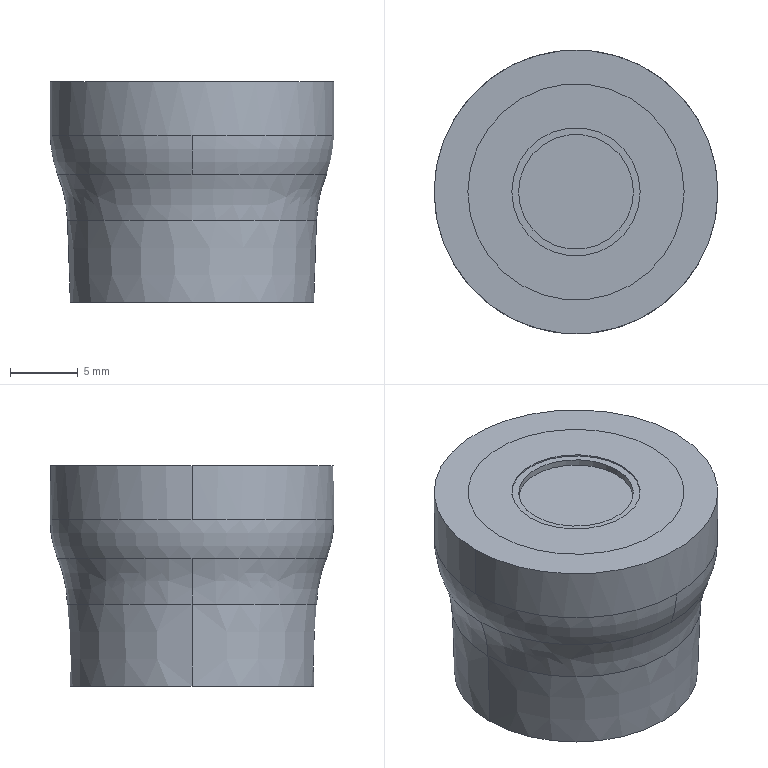Part | STEP file | TQ-DD-1105-THSensorMagnet1010_デフォルト | 3 solids | 119 faces | box 21 x 21 x 16.3 mm | volume 3743 mm3 | plane 62 | cylinder 36 | spline 10 | cone 9 | torus 2 | commonest cylinder face diameters 16 x8 13 x4 14 x4 18 x4 8.5 x2 9.5 x2